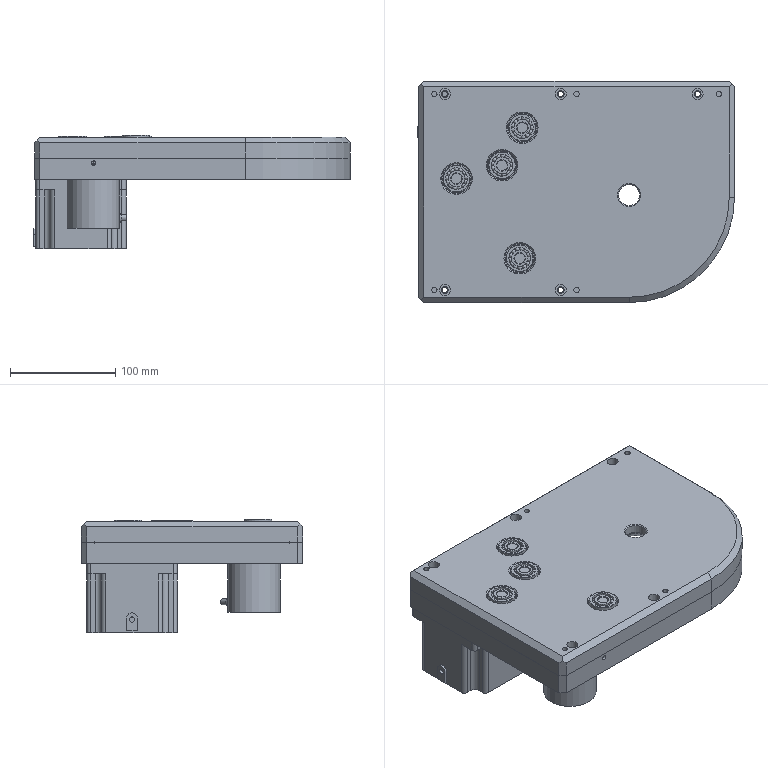Part | NX | features BREP 20 | 38 solids | 2566 faces | box 301 x 210 x 108 mm | volume 2303750 mm3 | cylinder 1810 | torus 286 | plane 277 | sphere 168 | cone 25 | commonest cylinder face diameters 24 x429 72 x242 56.248 x201 63 x200 176.248 x120 183 x120